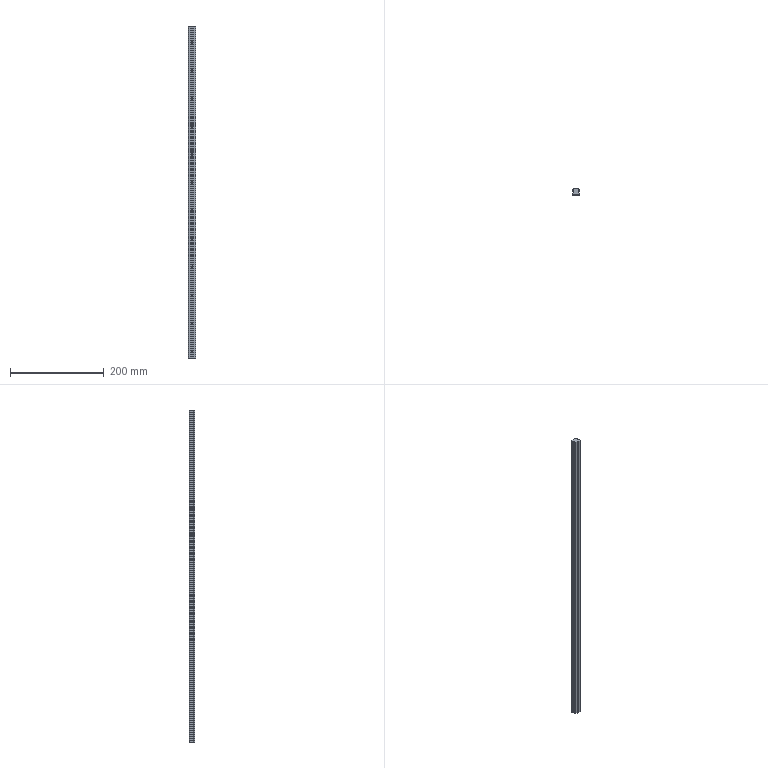Part | STEP file | 1 solid | 96 faces | box 15 x 12.5 x 710 mm | volume 113515 mm3 | cylinder 64 | plane 32 | commonest cylinder face diameters 3.5 x24 6 x24 0.6 x10 3 x4 1 x2